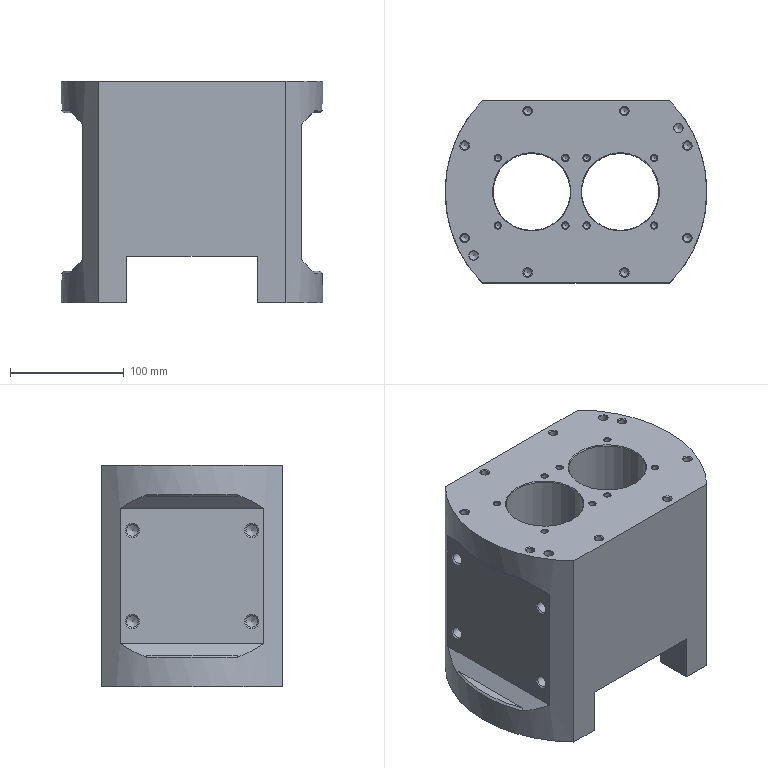NC program | NX | posted with a generic post | part box 230 x 160 x 195 mm
Lines 1426 to 1674 of 1674:
(PLANAR_MILL_COPY_COPY_COPY_COPY , TOOL : D6A45)
N2802 T07 M6
N2804 G54
N2806 G17 G0 G90 X-42.973 Y-72.476 B0. C0. S7500 M3
N2808 G43 Z30. H7
N2810 Z1.5
N2812 G94 G1 Z-1.5 F1250.
N2814 X-43.266 Y-73.393
N2816 G3 X-42.5 Y-73.75 R1.
N2818 X-39.75 Y-71. R2.75
N2820 X-42.5 Y-73.75 R-2.75
N2822 X-41.734 Y-73.393 R1.
N2824 G1 X-42.027 Y-72.476
N2826 Z1.5
N2828 G0 Z30.
N2830 X-90.473 Y-57.476
N2832 Z1.5
N2834 G1 Z-1.5
N2836 X-90.766 Y-58.393
N2838 G3 X-90. Y-58.75 R1.
N2840 X-87.25 Y-56. R2.75
N2842 X-90. Y-58.75 R-2.75
N2844 X-89.234 Y-58.393 R1.
N2846 G1 X-89.527 Y-57.476
N2848 Z1.5
N2850 G0 Z30.
N2852 X-99.407 Y-40.092
N2854 Z1.5
N2856 G1 Z-1.5
N2858 X-100.324 Y-39.798
N2860 G3 X-100.681 Y-40.564 R1.
N2862 X-97.931 Y-43.314 R2.75
N2864 X-100.681 Y-40.564 R-2.75
N2866 X-100.324 Y-41.33 R1.
N2868 G1 X-99.407 Y-41.037
N2870 Z1.5
N2872 G0 Z30.
N2874 X-69.18 Y-29.433
N2876 Z1.5
N2878 G1 Z-1.5
N2880 X-70.091 Y-28.932
N2882 G3 X-70.448 Y-29.698 R1.
N2884 X-68.698 Y-31.448 R1.75
N2886 X-70.448 Y-29.698 R-1.75
N2888 X-70.091 Y-30.465 R1.
N2890 G1 X-69.18 Y-29.964
N2892 Z1.5
N2894 G0 Z30.
N2896 X-70.731 Y1.503
N2898 Z1.5
N2900 G1 Z-1.5
N2902 X-71.609 Y0.766
N2904 G3 X-71.966 Y0. R1.
N2906 X-39. Y-32.966 R32.966
N2908 X-71.966 Y0. R-32.966
N2910 X-71.609 Y-0.766 R1.
N2912 G1 X-70.731 Y-1.503
N2914 Z1.5
N2916 G0 Z30.
N2918 X-9.567 Y-30.18
N2920 Z1.5
N2922 G1 Z-1.5
N2924 X-10.068 Y-31.091
N2926 G3 X-9.302 Y-31.448 R1.
N2928 X-7.552 Y-29.698 R1.75
N2930 X-9.302 Y-31.448 R-1.75
N2932 X-8.535 Y-31.091 R1.
N2934 G1 X-9.036 Y-30.18
N2936 Z1.5
N2938 G0 Z30.
N2940 X9.036
N2942 Z1.5
N2944 G1 Z-1.5
N2946 X8.535 Y-31.091
N2948 G3 X9.302 Y-31.448 R1.
N2950 X11.052 Y-29.698 R1.75
N2952 X9.302 Y-31.448 R-1.75
N2954 X10.068 Y-31.091 R1.
N2956 G1 X9.567 Y-30.18
N2958 Z1.5
N2960 G0 Z30.
N2962 X42.027 Y-72.476
N2964 Z1.5
N2966 G1 Z-1.5
N2968 X41.734 Y-73.393
N2970 G3 X42.5 Y-73.75 R1.
N2972 X45.25 Y-71. R2.75
N2974 X42.5 Y-73.75 R-2.75
N2976 X43.266 Y-73.393 R1.
N2978 G1 X42.973 Y-72.476
N2980 Z1.5
N2982 G0 Z30.
N2984 X99.407 Y-41.037
N2986 Z1.5
N2988 G1 Z-1.5
N2990 X100.324 Y-41.33
N2992 G3 X100.681 Y-40.564 R1.
N2994 X97.931 Y-37.814 R2.75
N2996 X100.681 Y-40.564 R-2.75
N2998 X100.324 Y-39.798 R1.
N3000 G1 X99.407 Y-40.092
N3002 Z1.5
N3004 G0 Z30.
N3006 X69.18 Y-29.964
N3008 Z1.5
N3010 G1 Z-1.5
N3012 X70.091 Y-30.465
N3014 G3 X70.448 Y-29.698 R1.
N3016 X68.698 Y-27.948 R1.75
N3018 X70.448 Y-29.698 R-1.75
N3020 X70.091 Y-28.932 R1.
N3022 G1 X69.18 Y-29.433
N3024 Z1.5
N3026 G0 Z30.
N3028 X70.731 Y-1.503
N3030 Z1.5
N3032 G1 Z-1.5
N3034 X71.609 Y-0.766
N3036 G3 X71.966 Y0. R1.
N3038 X39. Y32.966 R32.966
N3040 X71.966 Y0. R-32.966
N3042 X71.609 Y0.766 R1.
N3044 G1 X70.731 Y1.503
N3046 Z1.5
N3048 G0 Z30.
N3050 X69.18 Y29.433
N3052 Z1.5
N3054 G1 Z-1.5
N3056 X70.091 Y28.932
N3058 G3 X70.448 Y29.698 R1.
N3060 X68.698 Y31.448 R1.75
N3062 X70.448 Y29.698 R-1.75
N3064 X70.091 Y30.465 R1.
N3066 G1 X69.18 Y29.964
N3068 Z1.5
N3070 G0 Z30.
N3072 X99.407 Y40.092
N3074 Z1.5
N3076 G1 Z-1.5
N3078 X100.324 Y39.798
N3080 G3 X100.681 Y40.564 R1.
N3082 X97.931 Y43.314 R2.75
N3084 X100.681 Y40.564 R-2.75
N3086 X100.324 Y41.33 R1.
N3088 G1 X99.407 Y41.037
N3090 Z1.5
N3092 G0 Z30.
N3094 X91.476 Y55.527
N3096 Z1.5
N3098 G1 Z-1.5
N3100 X92.393 Y55.234
N3102 G3 X92.75 Y56. R1.
N3104 X90. Y58.75 R2.75
N3106 X92.75 Y56. R-2.75
N3108 X92.393 Y56.766 R1.
N3110 G1 X91.476 Y56.473
N3112 Z1.5
N3114 G0 Z30.
N3116 X42.973 Y72.476
N3118 Z1.5
N3120 G1 Z-1.5
N3122 X43.266 Y73.393
N3124 G3 X42.5 Y73.75 R1.
N3126 X39.75 Y71. R2.75
N3128 X42.5 Y73.75 R-2.75
N3130 X41.734 Y73.393 R1.
N3132 G1 X42.027 Y72.476
N3134 Z1.5
N3136 G0 Z30.
N3138 X9.567 Y30.18
N3140 Z1.5
N3142 G1 Z-1.5
N3144 X10.068 Y31.091
N3146 G3 X9.302 Y31.448 R1.
N3148 X7.552 Y29.698 R1.75
N3150 X9.302 Y31.448 R-1.75
N3152 X8.535 Y31.091 R1.
N3154 G1 X9.036 Y30.18
N3156 Z1.5
N3158 G0 Z30.
N3160 X-9.036
N3162 Z1.5
N3164 G1 Z-1.5
N3166 X-8.535 Y31.091
N3168 G3 X-9.302 Y31.448 R1.
N3170 X-11.052 Y29.698 R1.75
N3172 X-9.302 Y31.448 R-1.75
N3174 X-10.068 Y31.091 R1.
N3176 G1 X-9.567 Y30.18
N3178 Z1.5
N3180 G0 Z30.
N3182 X-42.027 Y72.476
N3184 Z1.5
N3186 G1 Z-1.5
N3188 X-41.734 Y73.393
N3190 G3 X-42.5 Y73.75 R1.
N3192 X-45.25 Y71. R2.75
N3194 X-42.5 Y73.75 R-2.75
N3196 X-43.266 Y73.393 R1.
N3198 G1 X-42.973 Y72.476
N3200 Z1.5
N3202 G0 Z30.
N3204 X-69.18 Y29.964
N3206 Z1.5
N3208 G1 Z-1.5
N3210 X-70.091 Y30.465
N3212 G3 X-70.448 Y29.698 R1.
N3214 X-68.698 Y27.948 R1.75
N3216 X-70.448 Y29.698 R-1.75
N3218 X-70.091 Y28.932 R1.
N3220 G1 X-69.18 Y29.433
N3222 Z1.5
N3224 G0 Z30.
N3226 X-99.407 Y41.037
N3228 Z1.5
N3230 G1 Z-1.5
N3232 X-100.324 Y41.33
N3234 G3 X-100.681 Y40.564 R1.
N3236 X-97.931 Y37.814 R2.75
N3238 X-100.681 Y40.564 R-2.75
N3240 X-100.324 Y39.798 R1.
N3242 G1 X-99.407 Y40.092
N3244 Z1.5
N3246 G0 Z30.
(PLANAR_MILL_COPY_COPY_COPY_COPY_COPY , TOOL : D6A45)
N3248 X1.473 Y-82.5
N3250 Z1.5
N3252 G1 Z-1.5
N3254 X0.766 Y-81.657
N3256 G3 X0. Y-81.3 R1.
N3258 G1 X-82.529
N3260 G2 X-83.607 Y-80.843 R1.5
N3262 X-83.607 Y80.843 R116.3
N3264 X-82.529 Y81.3 R1.5
N3266 G1 X82.529
N3268 G2 X83.607 Y80.843 R1.5
N3270 X83.607 Y-80.843 R116.3
N3272 X82.529 Y-81.3 R1.5
N3274 G1 X0.
N3276 G3 X-0.766 Y-81.657 R1.
N3278 G1 X-1.473 Y-82.5
N3280 Z1.5
N3282 G0 Z30.
N3284 M5
N3286 M2